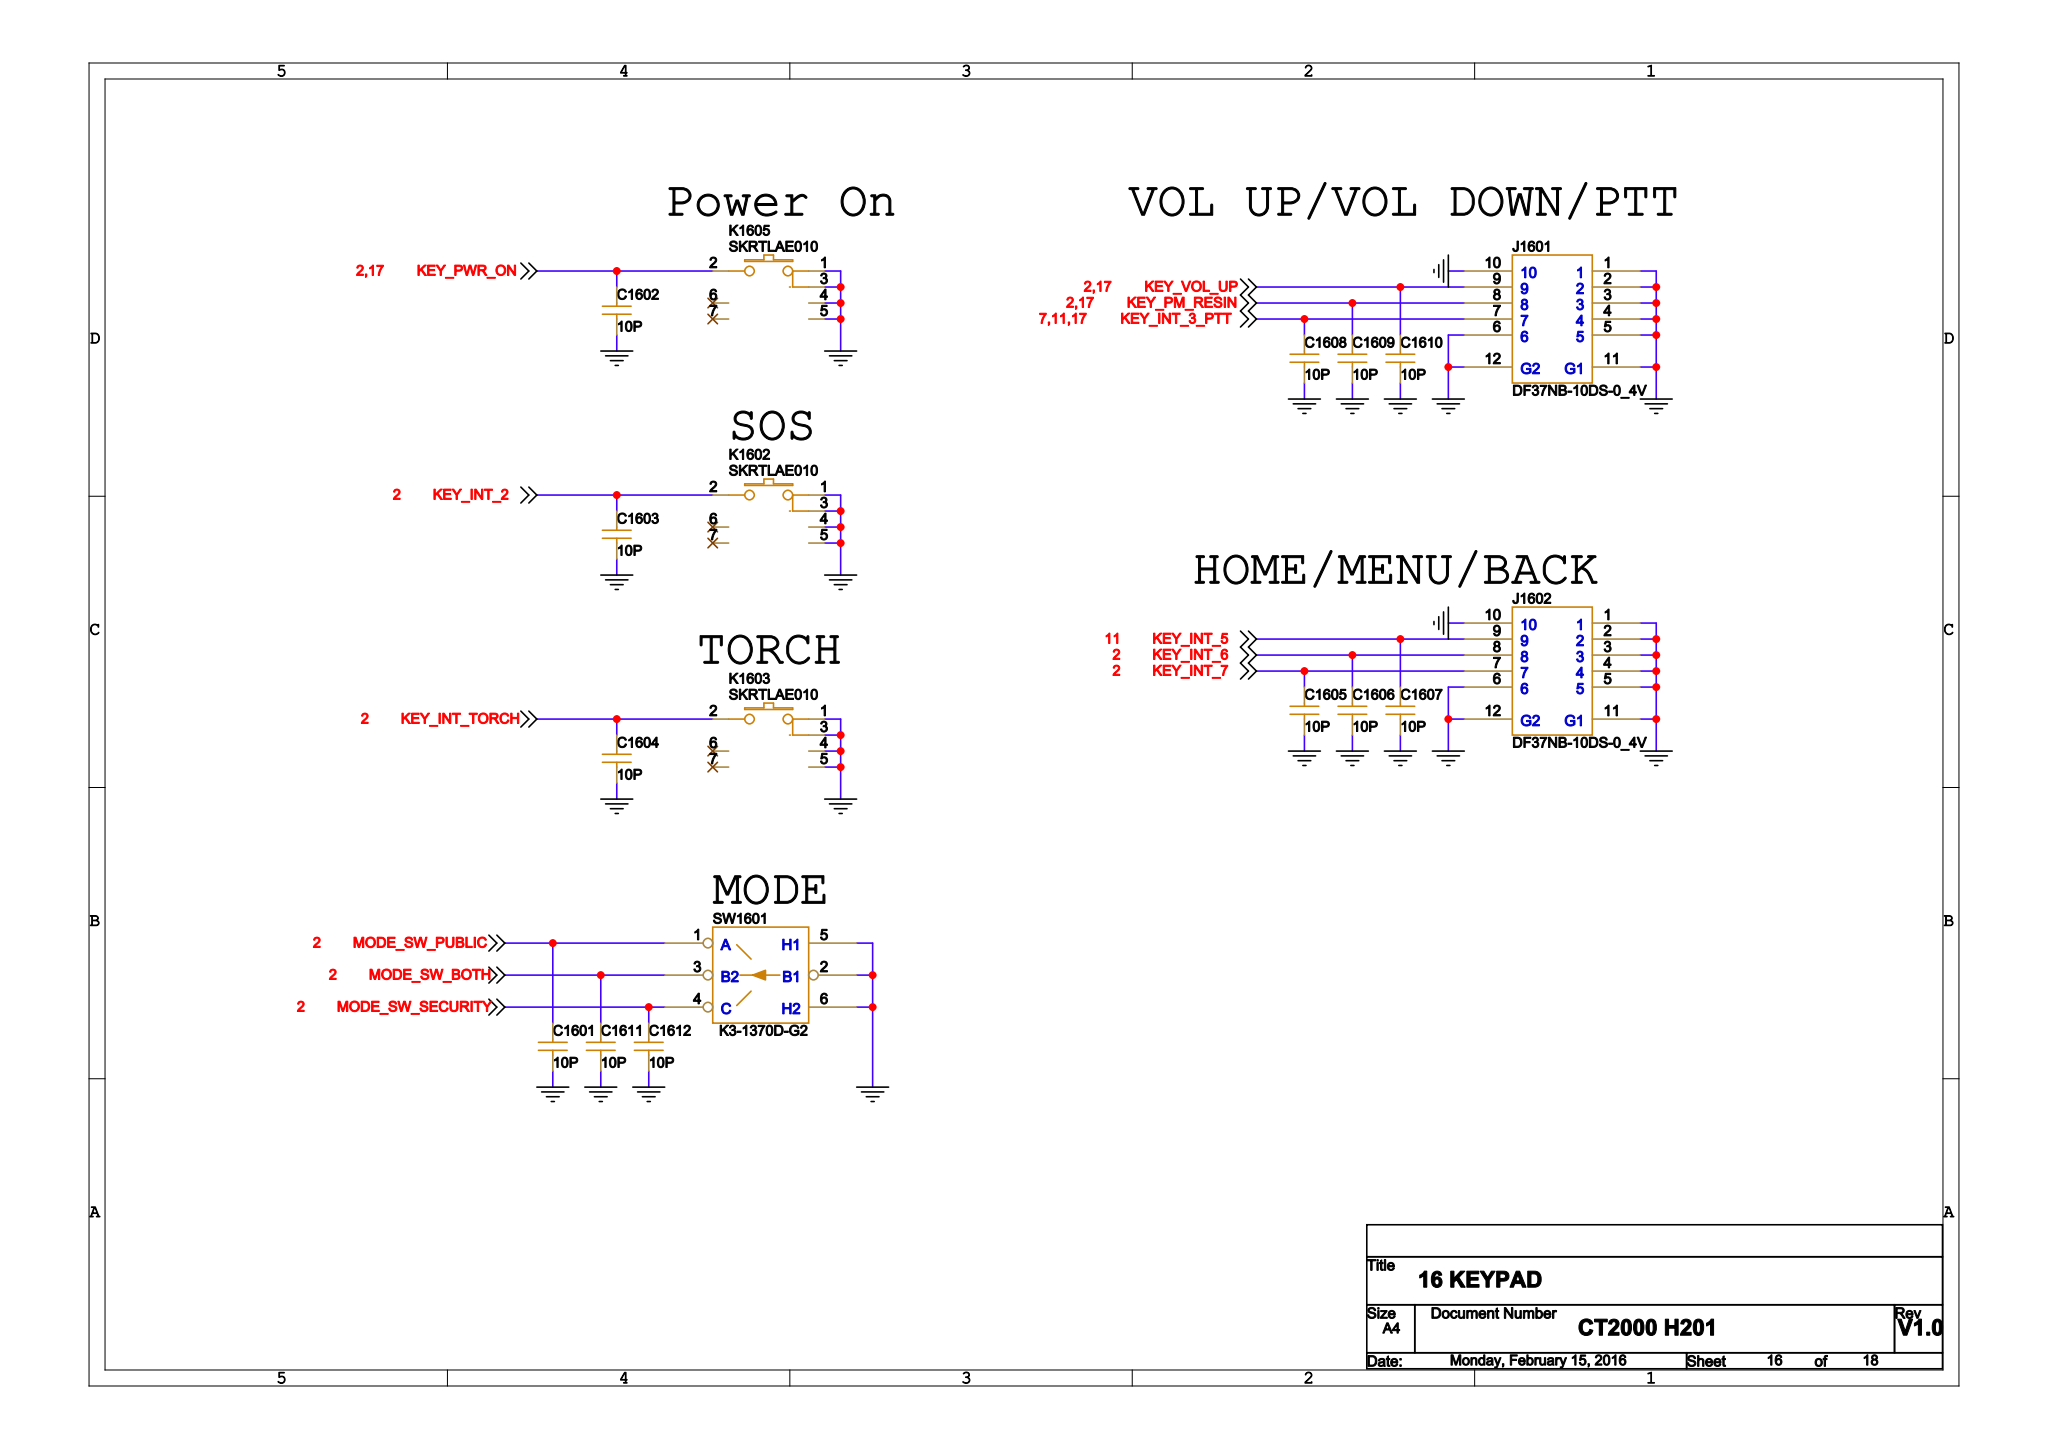Circuit board | Cadence Allegro | 573 parts | 376 nets | one sheet of the schematic
Parts on this sheet (reference | value | footprint):
C1601 | 10P | C0402
C1602 | 10P | C0402
C1603 | 10P | C0402
C1604 | 10P | C0402
C1605 | 10P | C0402
C1606 | 10P | C0402
C1607 | 10P | C0402
C1608 | 10P | C0402
C1609 | 10P | C0402
C1610 | 10P | C0402
C1611 | 10P | C0402
C1612 | 10P | C0402
J1601 | DF37NB-10DS-0_4V | BTB_DF37NB-10DS-0_4V_CW
J1602 | DF37NB-10DS-0_4V | BTB_DF37NB-10DS-0_4V_CW
K1602 | SKRTLAE010 | KEY_SKRTLAE010
K1603 | SKRTLAE010 | KEY_SKRTLAE010
K1605 | SKRTLAE010 | KEY_SKRTLAE010
SW1601 | K3-1370D-G2 | TOGGLE_SW_K3-1370D-G2
Nets of these parts (net: part-pin ...):
GND: C1601-2 C1602-2 C1603-2 C1604-2 C1605-2 C1606-2 C1607-2 C1608-2 C1609-2 C1610-2 C1611-2 C1612-2 J1601-1 J1601-2 J1601-3 J1601-4 J1601-5 J1601-6 J1601-10 J1601-11 J1601-12 J1602-1 J1602-2 J1602-3 J1602-4 J1602-5 J1602-6 J1602-10 J1602-11 J1602-12 K1602-1 K1602-3 K1602-4 K1602-5 K1603-1 K1603-3 K1603-4 K1603-5 K1605-1 K1605-3 K1605-4 K1605-5 SW1601-2 SW1601-5 SW1601-6
KEY_INT_3_PTT: C1608-1 J1601-7
KEY_PM_RESIN: C1609-1 J1601-8
KEY_VOL_UP: C1610-1 J1601-9
KEY_INT_7: C1605-1 J1602-7
KEY_INT_6: C1606-1 J1602-8
KEY_INT_5: C1607-1 J1602-9
KEY_INT_2: C1603-1 K1602-2
KEY_INT_TORCH: C1604-1 K1603-2
KEY_PWR_ON: C1602-1 K1605-2
MODE_SW_PUBLIC: C1601-1 SW1601-1
MODE_SW_BOTH: C1611-1 SW1601-3
MODE_SW_SECURITY: C1612-1 SW1601-4